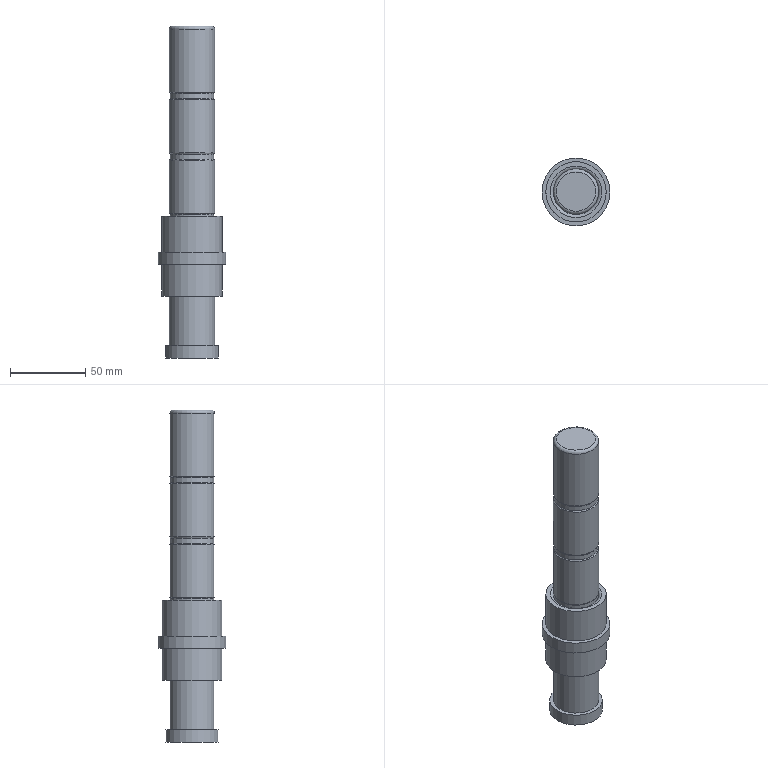Part | STEP file | EGP | 2 solids | 42 faces | box 45 x 45 x 220 mm | volume 186041 mm3 | cylinder 17 | plane 11 | torus 11 | cone 3 | commonest cylinder face diameters 30 x6 29 x4 40 x2 10.2 x1 11.96 x1 12 x1